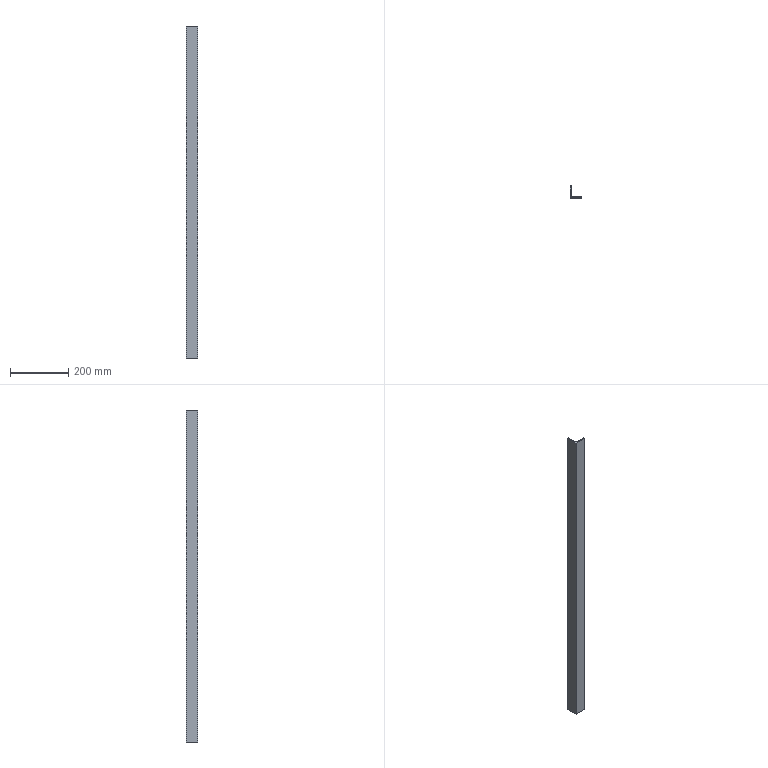Part | SolidWorks | features Extrusion 1 | 1 solid | 11 faces | box 40 x 40 x 1138 mm | volume 352057 mm3 | plane 8 | cylinder 3 | commonest cylinder face diameters 0.02 x2 10 x1
STEP:
#1=CARTESIAN_POINT('',(0.,0.,0.));
#2=VERTEX_POINT('',#1);
#3=CARTESIAN_POINT('',(40.,0.,0.));
#4=VERTEX_POINT('',#3);
#5=CARTESIAN_POINT('',(40.,0.,0.));
#6=DIRECTION('',(1.,0.,0.));
#7=VECTOR('',#6,1000.);
#8=LINE('',#5,#7);
#9=EDGE_CURVE('',#2,#4,#8,.T.);
#10=ORIENTED_EDGE('',*,*,#9,.T.);
#11=CARTESIAN_POINT('',(40.,0.,1138.));
#12=VERTEX_POINT('',#11);
#13=CARTESIAN_POINT('',(40.,0.,1138.));
#14=DIRECTION('',(0.,0.,-1.));
#15=VECTOR('',#14,1000.);
#16=LINE('',#13,#15);
#17=EDGE_CURVE('',#12,#4,#16,.T.);
#18=ORIENTED_EDGE('',*,*,#17,.F.);
#19=CARTESIAN_POINT('',(0.,0.,1138.));
#20=VERTEX_POINT('',#19);
#21=CARTESIAN_POINT('',(40.,0.,1138.));
#22=DIRECTION('',(1.,0.,0.));
#23=VECTOR('',#22,1000.);
#24=LINE('',#21,#23);
#25=EDGE_CURVE('',#20,#12,#24,.T.);
#26=ORIENTED_EDGE('',*,*,#25,.F.);
#27=CARTESIAN_POINT('',(0.,0.,1138.));
#28=DIRECTION('',(0.,0.,-1.));
#29=VECTOR('',#28,1000.);
#30=LINE('',#27,#29);
#31=EDGE_CURVE('',#20,#2,#30,.T.);
#32=ORIENTED_EDGE('',*,*,#31,.T.);
#33=EDGE_LOOP('',(#10,#18,#26,#32));
#34=FACE_OUTER_BOUND('',#33,.T.);
#35=CARTESIAN_POINT('',(40.,0.,1138.));
#36=DIRECTION('',(0.,1.,0.));
#37=DIRECTION('',(-1.,0.,0.));
#38=AXIS2_PLACEMENT_3D('',#35,#36,#37);
#39=PLANE('',#38);
#40=ADVANCED_FACE('',(#34),#39,.F.);
#41=CARTESIAN_POINT('',(40.,3.99,0.));
#42=VERTEX_POINT('',#41);
#43=CARTESIAN_POINT('',(40.,3.99,0.));
#44=DIRECTION('',(0.,1.,0.));
#45=VECTOR('',#44,1000.);
#46=LINE('',#43,#45);
#47=EDGE_CURVE('',#4,#42,#46,.T.);
#48=ORIENTED_EDGE('',*,*,#47,.T.);
#49=CARTESIAN_POINT('',(40.,3.99,1138.));
#50=VERTEX_POINT('',#49);
#51=CARTESIAN_POINT('',(40.,3.99,1138.));
#52=DIRECTION('',(0.,0.,-1.));
#53=VECTOR('',#52,1000.);
#54=LINE('',#51,#53);
#55=EDGE_CURVE('',#50,#42,#54,.T.);
#56=ORIENTED_EDGE('',*,*,#55,.F.);
#57=CARTESIAN_POINT('',(40.,3.99,1138.));
#58=DIRECTION('',(0.,1.,0.));
#59=VECTOR('',#58,1000.);
#60=LINE('',#57,#59);
#61=EDGE_CURVE('',#12,#50,#60,.T.);
#62=ORIENTED_EDGE('',*,*,#61,.F.);
#63=ORIENTED_EDGE('',*,*,#17,.T.);
#64=EDGE_LOOP('',(#48,#56,#62,#63));
#65=FACE_OUTER_BOUND('',#64,.T.);
#66=CARTESIAN_POINT('',(40.,3.99,1138.));
#67=DIRECTION('',(-1.,0.,0.));
#68=DIRECTION('',(0.,-1.,0.));
#69=AXIS2_PLACEMENT_3D('',#66,#67,#68);
#70=PLANE('',#69);
#71=ADVANCED_FACE('',(#65),#70,.F.);
#72=CARTESIAN_POINT('',(39.99,4.,0.));
#73=VERTEX_POINT('',#72);
#74=CARTESIAN_POINT('',(39.99,3.99,0.));
#75=DIRECTION('',(0.,0.,1.));
#76=DIRECTION('',(1.,0.,0.));
#77=AXIS2_PLACEMENT_3D('',#74,#75,#76);
#78=CIRCLE('',#77,0.01);
#79=EDGE_CURVE('',#42,#73,#78,.T.);
#80=ORIENTED_EDGE('',*,*,#79,.T.);
#81=CARTESIAN_POINT('',(39.99,4.,1138.));
#82=VERTEX_POINT('',#81);
#83=CARTESIAN_POINT('',(39.99,4.,1138.));
#84=DIRECTION('',(0.,0.,-1.));
#85=VECTOR('',#84,1000.);
#86=LINE('',#83,#85);
#87=EDGE_CURVE('',#82,#73,#86,.T.);
#88=ORIENTED_EDGE('',*,*,#87,.F.);
#89=CARTESIAN_POINT('',(39.99,3.99,1138.));
#90=DIRECTION('',(0.,0.,1.));
#91=DIRECTION('',(1.,0.,0.));
#92=AXIS2_PLACEMENT_3D('',#89,#90,#91);
#93=CIRCLE('',#92,0.01);
#94=EDGE_CURVE('',#50,#82,#93,.T.);
#95=ORIENTED_EDGE('',*,*,#94,.F.);
#96=ORIENTED_EDGE('',*,*,#55,.T.);
#97=EDGE_LOOP('',(#80,#88,#95,#96));
#98=FACE_OUTER_BOUND('',#97,.T.);
#99=CARTESIAN_POINT('',(39.99,3.99,1138.));
#100=DIRECTION('',(0.,0.,-1.));
#101=DIRECTION('',(-1.,0.,0.));
#102=AXIS2_PLACEMENT_3D('',#99,#100,#101);
#103=CYLINDRICAL_SURFACE('',#102,0.01);
#104=ADVANCED_FACE('',(#98),#103,.T.);
#105=CARTESIAN_POINT('',(9.,4.,0.));
#106=VERTEX_POINT('',#105);
#107=CARTESIAN_POINT('',(9.,4.,0.));
#108=DIRECTION('',(-1.,0.,0.));
#109=VECTOR('',#108,1000.);
#110=LINE('',#107,#109);
#111=EDGE_CURVE('',#73,#106,#110,.T.);
#112=ORIENTED_EDGE('',*,*,#111,.T.);
#113=CARTESIAN_POINT('',(9.,4.,1138.));
#114=VERTEX_POINT('',#113);
#115=CARTESIAN_POINT('',(9.,4.,1138.));
#116=DIRECTION('',(0.,0.,-1.));
#117=VECTOR('',#116,1000.);
#118=LINE('',#115,#117);
#119=EDGE_CURVE('',#114,#106,#118,.T.);
#120=ORIENTED_EDGE('',*,*,#119,.F.);
#121=CARTESIAN_POINT('',(9.,4.,1138.));
#122=DIRECTION('',(-1.,0.,0.));
#123=VECTOR('',#122,1000.);
#124=LINE('',#121,#123);
#125=EDGE_CURVE('',#82,#114,#124,.T.);
#126=ORIENTED_EDGE('',*,*,#125,.F.);
#127=ORIENTED_EDGE('',*,*,#87,.T.);
#128=EDGE_LOOP('',(#112,#120,#126,#127));
#129=FACE_OUTER_BOUND('',#128,.T.);
#130=CARTESIAN_POINT('',(9.,4.,1138.));
#131=DIRECTION('',(0.,-1.,0.));
#132=DIRECTION('',(1.,0.,0.));
#133=AXIS2_PLACEMENT_3D('',#130,#131,#132);
#134=PLANE('',#133);
#135=ADVANCED_FACE('',(#129),#134,.F.);
#136=CARTESIAN_POINT('',(4.,9.,0.));
#137=VERTEX_POINT('',#136);
#138=CARTESIAN_POINT('',(9.,9.,0.));
#139=DIRECTION('',(0.,0.,-1.));
#140=DIRECTION('',(-1.,0.,0.));
#141=AXIS2_PLACEMENT_3D('',#138,#139,#140);
#142=CIRCLE('',#141,5.);
#143=EDGE_CURVE('',#106,#137,#142,.T.);
#144=ORIENTED_EDGE('',*,*,#143,.T.);
#145=CARTESIAN_POINT('',(4.,9.,1138.));
#146=VERTEX_POINT('',#145);
#147=CARTESIAN_POINT('',(4.,9.,1138.));
#148=DIRECTION('',(0.,0.,-1.));
#149=VECTOR('',#148,1000.);
#150=LINE('',#147,#149);
#151=EDGE_CURVE('',#146,#137,#150,.T.);
#152=ORIENTED_EDGE('',*,*,#151,.F.);
#153=CARTESIAN_POINT('',(9.,9.,1138.));
#154=DIRECTION('',(0.,0.,-1.));
#155=DIRECTION('',(-1.,0.,0.));
#156=AXIS2_PLACEMENT_3D('',#153,#154,#155);
#157=CIRCLE('',#156,5.);
#158=EDGE_CURVE('',#114,#146,#157,.T.);
#159=ORIENTED_EDGE('',*,*,#158,.F.);
#160=ORIENTED_EDGE('',*,*,#119,.T.);
#161=EDGE_LOOP('',(#144,#152,#159,#160));
#162=FACE_OUTER_BOUND('',#161,.T.);
#163=CARTESIAN_POINT('',(9.,9.,1138.));
#164=DIRECTION('',(0.,0.,-1.));
#165=DIRECTION('',(-1.,0.,0.));
#166=AXIS2_PLACEMENT_3D('',#163,#164,#165);
#167=CYLINDRICAL_SURFACE('',#166,5.);
#168=ADVANCED_FACE('',(#162),#167,.F.);
#169=CARTESIAN_POINT('',(4.,39.99,0.));
#170=VERTEX_POINT('',#169);
#171=CARTESIAN_POINT('',(4.,39.99,0.));
#172=DIRECTION('',(0.,1.,0.));
#173=VECTOR('',#172,1000.);
#174=LINE('',#171,#173);
#175=EDGE_CURVE('',#137,#170,#174,.T.);
#176=ORIENTED_EDGE('',*,*,#175,.T.);
#177=CARTESIAN_POINT('',(4.,39.99,1138.));
#178=VERTEX_POINT('',#177);
#179=CARTESIAN_POINT('',(4.,39.99,1138.));
#180=DIRECTION('',(0.,0.,-1.));
#181=VECTOR('',#180,1000.);
#182=LINE('',#179,#181);
#183=EDGE_CURVE('',#178,#170,#182,.T.);
#184=ORIENTED_EDGE('',*,*,#183,.F.);
#185=CARTESIAN_POINT('',(4.,39.99,1138.));
#186=DIRECTION('',(0.,1.,0.));
#187=VECTOR('',#186,1000.);
#188=LINE('',#185,#187);
#189=EDGE_CURVE('',#146,#178,#188,.T.);
#190=ORIENTED_EDGE('',*,*,#189,.F.);
#191=ORIENTED_EDGE('',*,*,#151,.T.);
#192=EDGE_LOOP('',(#176,#184,#190,#191));
#193=FACE_OUTER_BOUND('',#192,.T.);
#194=CARTESIAN_POINT('',(4.,39.99,1138.));
#195=DIRECTION('',(-1.,0.,0.));
#196=DIRECTION('',(0.,-1.,0.));
#197=AXIS2_PLACEMENT_3D('',#194,#195,#196);
#198=PLANE('',#197);
#199=ADVANCED_FACE('',(#193),#198,.F.);
#200=CARTESIAN_POINT('',(3.99,40.,0.));
#201=VERTEX_POINT('',#200);
#202=CARTESIAN_POINT('',(3.99,39.99,0.));
#203=DIRECTION('',(0.,0.,1.));
#204=DIRECTION('',(1.,0.,0.));
#205=AXIS2_PLACEMENT_3D('',#202,#203,#204);
#206=CIRCLE('',#205,0.01);
#207=EDGE_CURVE('',#170,#201,#206,.T.);
#208=ORIENTED_EDGE('',*,*,#207,.T.);
#209=CARTESIAN_POINT('',(3.99,40.,1138.));
#210=VERTEX_POINT('',#209);
#211=CARTESIAN_POINT('',(3.99,40.,1138.));
#212=DIRECTION('',(0.,0.,-1.));
#213=VECTOR('',#212,1000.);
#214=LINE('',#211,#213);
#215=EDGE_CURVE('',#210,#201,#214,.T.);
#216=ORIENTED_EDGE('',*,*,#215,.F.);
#217=CARTESIAN_POINT('',(3.99,39.99,1138.));
#218=DIRECTION('',(0.,0.,1.));
#219=DIRECTION('',(1.,0.,0.));
#220=AXIS2_PLACEMENT_3D('',#217,#218,#219);
#221=CIRCLE('',#220,0.01);
#222=EDGE_CURVE('',#178,#210,#221,.T.);
#223=ORIENTED_EDGE('',*,*,#222,.F.);
#224=ORIENTED_EDGE('',*,*,#183,.T.);
#225=EDGE_LOOP('',(#208,#216,#223,#224));
#226=FACE_OUTER_BOUND('',#225,.T.);
#227=CARTESIAN_POINT('',(3.99,39.99,1138.));
#228=DIRECTION('',(0.,0.,-1.));
#229=DIRECTION('',(-1.,0.,0.));
#230=AXIS2_PLACEMENT_3D('',#227,#228,#229);
#231=CYLINDRICAL_SURFACE('',#230,0.01);
#232=ADVANCED_FACE('',(#226),#231,.T.);
#233=CARTESIAN_POINT('',(0.,40.,0.));
#234=VERTEX_POINT('',#233);
#235=CARTESIAN_POINT('',(0.,40.,0.));
#236=DIRECTION('',(-1.,0.,0.));
#237=VECTOR('',#236,1000.);
#238=LINE('',#235,#237);
#239=EDGE_CURVE('',#201,#234,#238,.T.);
#240=ORIENTED_EDGE('',*,*,#239,.T.);
#241=CARTESIAN_POINT('',(0.,40.,1138.));
#242=VERTEX_POINT('',#241);
#243=CARTESIAN_POINT('',(0.,40.,1138.));
#244=DIRECTION('',(0.,0.,-1.));
#245=VECTOR('',#244,1000.);
#246=LINE('',#243,#245);
#247=EDGE_CURVE('',#242,#234,#246,.T.);
#248=ORIENTED_EDGE('',*,*,#247,.F.);
#249=CARTESIAN_POINT('',(0.,40.,1138.));
#250=DIRECTION('',(-1.,0.,0.));
#251=VECTOR('',#250,1000.);
#252=LINE('',#249,#251);
#253=EDGE_CURVE('',#210,#242,#252,.T.);
#254=ORIENTED_EDGE('',*,*,#253,.F.);
#255=ORIENTED_EDGE('',*,*,#215,.T.);
#256=EDGE_LOOP('',(#240,#248,#254,#255));
#257=FACE_OUTER_BOUND('',#256,.T.);
#258=CARTESIAN_POINT('',(0.,40.,1138.));
#259=DIRECTION('',(0.,-1.,0.));
#260=DIRECTION('',(0.,0.,-1.));
#261=AXIS2_PLACEMENT_3D('',#258,#259,#260);
#262=PLANE('',#261);
#263=ADVANCED_FACE('',(#257),#262,.F.);
#264=CARTESIAN_POINT('',(0.,0.,0.));
#265=DIRECTION('',(0.,-1.,0.));
#266=VECTOR('',#265,1000.);
#267=LINE('',#264,#266);
#268=EDGE_CURVE('',#234,#2,#267,.T.);
#269=ORIENTED_EDGE('',*,*,#268,.T.);
#270=ORIENTED_EDGE('',*,*,#31,.F.);
#271=CARTESIAN_POINT('',(0.,0.,1138.));
#272=DIRECTION('',(0.,-1.,0.));
#273=VECTOR('',#272,1000.);
#274=LINE('',#271,#273);
#275=EDGE_CURVE('',#242,#20,#274,.T.);
#276=ORIENTED_EDGE('',*,*,#275,.F.);
#277=ORIENTED_EDGE('',*,*,#247,.T.);
#278=EDGE_LOOP('',(#269,#270,#276,#277));
#279=FACE_OUTER_BOUND('',#278,.T.);
#280=CARTESIAN_POINT('',(0.,0.,1138.));
#281=DIRECTION('',(1.,0.,0.));
#282=DIRECTION('',(0.,0.,-1.));
#283=AXIS2_PLACEMENT_3D('',#280,#281,#282);
#284=PLANE('',#283);
#285=ADVANCED_FACE('',(#279),#284,.F.);
#286=ORIENTED_EDGE('',*,*,#25,.T.);
#287=ORIENTED_EDGE('',*,*,#61,.T.);
#288=ORIENTED_EDGE('',*,*,#94,.T.);
#289=ORIENTED_EDGE('',*,*,#125,.T.);
#290=ORIENTED_EDGE('',*,*,#158,.T.);
#291=ORIENTED_EDGE('',*,*,#189,.T.);
#292=ORIENTED_EDGE('',*,*,#222,.T.);
#293=ORIENTED_EDGE('',*,*,#253,.T.);
#294=ORIENTED_EDGE('',*,*,#275,.T.);
#295=EDGE_LOOP('',(#286,#287,#288,#289,#290,#291,#292,#293,#294));
#296=FACE_OUTER_BOUND('',#295,.T.);
#297=CARTESIAN_POINT('',(3.99,39.99,1138.));
#298=DIRECTION('',(0.,0.,1.));
#299=DIRECTION('',(1.,0.,0.));
#300=AXIS2_PLACEMENT_3D('',#297,#298,#299);
#301=PLANE('',#300);
#302=ADVANCED_FACE('',(#296),#301,.T.);
#303=ORIENTED_EDGE('',*,*,#9,.F.);
#304=ORIENTED_EDGE('',*,*,#268,.F.);
#305=ORIENTED_EDGE('',*,*,#239,.F.);
#306=ORIENTED_EDGE('',*,*,#207,.F.);
#307=ORIENTED_EDGE('',*,*,#175,.F.);
#308=ORIENTED_EDGE('',*,*,#143,.F.);
#309=ORIENTED_EDGE('',*,*,#111,.F.);
#310=ORIENTED_EDGE('',*,*,#79,.F.);
#311=ORIENTED_EDGE('',*,*,#47,.F.);
#312=EDGE_LOOP('',(#303,#304,#305,#306,#307,#308,#309,#310,#311));
#313=FACE_OUTER_BOUND('',#312,.T.);
#314=CARTESIAN_POINT('',(3.99,39.99,0.));
#315=DIRECTION('',(0.,0.,1.));
#316=DIRECTION('',(1.,0.,0.));
#317=AXIS2_PLACEMENT_3D('',#314,#315,#316);
#318=PLANE('',#317);
#319=ADVANCED_FACE('',(#313),#318,.F.);
#320=CLOSED_SHELL('',(#40,#71,#104,#135,#168,#199,#232,#263,#285,#302,#319));
#321=MANIFOLD_SOLID_BREP('',#320);
#322=CARTESIAN_POINT('',(0.,0.,0.));
#323=DIRECTION('',(0.,0.,1.));
#324=DIRECTION('',(1.,0.,0.));
#325=AXIS2_PLACEMENT_3D('',#322,#323,#324);
#326=(LENGTH_UNIT()NAMED_UNIT(*)SI_UNIT(.MILLI.,.METRE.));
#327=UNCERTAINTY_MEASURE_WITH_UNIT(LENGTH_MEASURE(0.00001),#326,'','');
#328=(NAMED_UNIT(*)PLANE_ANGLE_UNIT()SI_UNIT($,.RADIAN.));
#329=(NAMED_UNIT(*)SI_UNIT($,.STERADIAN.)SOLID_ANGLE_UNIT());
#330=(GEOMETRIC_REPRESENTATION_CONTEXT(3)GLOBAL_UNCERTAINTY_ASSIGNED_CONTEXT((#327))GLOBAL_UNIT_ASSIGNED_CONTEXT((#326,#328,#329))REPRESENTATION_CONTEXT('',''));
#331=ADVANCED_BREP_SHAPE_REPRESENTATION('',(#321,#325),#330);